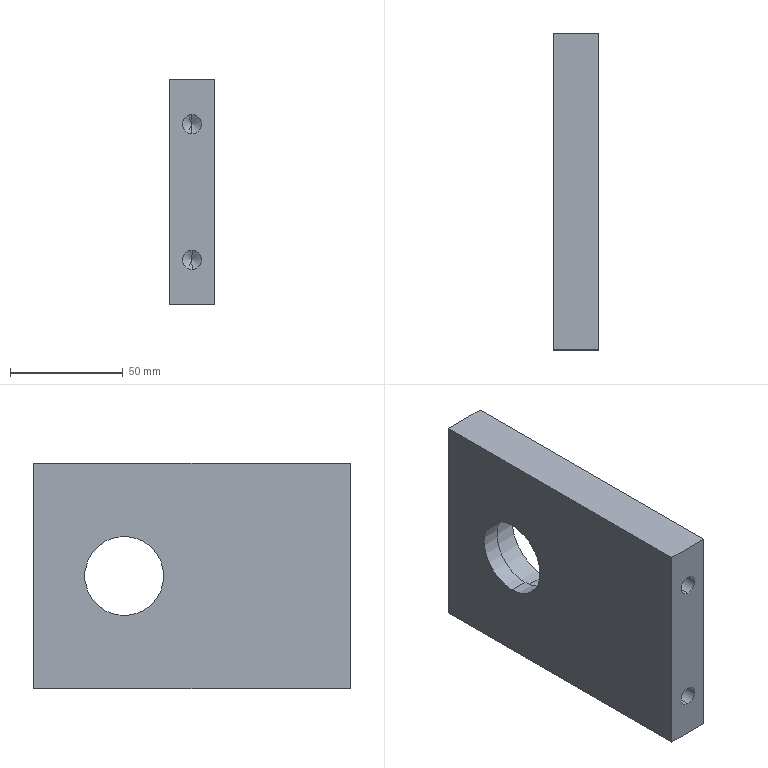Part | SolidWorks | features HoleWzd 2, ICE 2, Extrusion 1 | 1 solid | 27 faces | box 20 x 140 x 100 mm | volume 253738 mm3 | cylinder 12 | cone 8 | plane 7 | commonest cylinder face diameters 5 x4 8.5 x4 35 x2 40 x2
STEP:
#1=CARTESIAN_POINT('',(10.,55.,-32.5));
#2=VERTEX_POINT('',#1);
#3=CARTESIAN_POINT('',(10.,55.,-27.5));
#4=VERTEX_POINT('',#3);
#5=CARTESIAN_POINT('',(10.,55.,-30.));
#6=DIRECTION('',(0.,1.,0.));
#7=DIRECTION('',(0.,0.,1.));
#8=AXIS2_PLACEMENT_3D('',#5,#6,#7);
#9=CIRCLE('',#8,2.5);
#10=EDGE_CURVE('',#2,#4,#9,.T.);
#11=ORIENTED_EDGE('',*,*,#10,.F.);
#12=CARTESIAN_POINT('',(10.,70.,-32.5));
#13=VERTEX_POINT('',#12);
#14=CARTESIAN_POINT('',(10.,70.,-32.5));
#15=DIRECTION('',(0.,1.,0.));
#16=VECTOR('',#15,1000.);
#17=LINE('',#14,#16);
#18=EDGE_CURVE('',#2,#13,#17,.T.);
#19=ORIENTED_EDGE('',*,*,#18,.T.);
#20=CARTESIAN_POINT('',(10.,70.,-27.5));
#21=VERTEX_POINT('',#20);
#22=CARTESIAN_POINT('',(10.,70.,-30.));
#23=DIRECTION('',(0.,1.,0.));
#24=DIRECTION('',(0.,0.,1.));
#25=AXIS2_PLACEMENT_3D('',#22,#23,#24);
#26=CIRCLE('',#25,2.5);
#27=EDGE_CURVE('',#13,#21,#26,.T.);
#28=ORIENTED_EDGE('',*,*,#27,.T.);
#29=CARTESIAN_POINT('',(10.,70.,-27.5));
#30=DIRECTION('',(0.,1.,0.));
#31=VECTOR('',#30,1000.);
#32=LINE('',#29,#31);
#33=EDGE_CURVE('',#4,#21,#32,.T.);
#34=ORIENTED_EDGE('',*,*,#33,.F.);
#35=EDGE_LOOP('',(#11,#19,#28,#34));
#36=FACE_OUTER_BOUND('',#35,.T.);
#37=CARTESIAN_POINT('',(10.,70.,-30.));
#38=DIRECTION('',(0.,1.,0.));
#39=DIRECTION('',(0.,0.,1.));
#40=AXIS2_PLACEMENT_3D('',#37,#38,#39);
#41=CYLINDRICAL_SURFACE('',#40,2.5);
#42=ADVANCED_FACE('',(#36),#41,.F.);
#43=CARTESIAN_POINT('',(10.,53.498,-30.));
#44=VERTEX_POINT('',#43);
#45=CARTESIAN_POINT('',(10.,55.,-27.5));
#46=DIRECTION('',(0.,0.515,0.8572));
#47=VECTOR('',#46,1000.);
#48=LINE('',#45,#47);
#49=EDGE_CURVE('',#44,#4,#48,.T.);
#50=ORIENTED_EDGE('',*,*,#49,.F.);
#51=CARTESIAN_POINT('',(10.,55.,-32.5));
#52=DIRECTION('',(0.,0.515,-0.8572));
#53=VECTOR('',#52,1000.);
#54=LINE('',#51,#53);
#55=EDGE_CURVE('',#44,#2,#54,.T.);
#56=ORIENTED_EDGE('',*,*,#55,.T.);
#57=ORIENTED_EDGE('',*,*,#10,.T.);
#58=EDGE_LOOP('',(#50,#56,#57));
#59=FACE_OUTER_BOUND('',#58,.T.);
#60=CARTESIAN_POINT('',(10.,55.,-30.));
#61=DIRECTION('',(0.,1.,0.));
#62=DIRECTION('',(0.,0.,1.));
#63=AXIS2_PLACEMENT_3D('',#60,#61,#62);
#64=CONICAL_SURFACE('',#63,2.5,1.03);
#65=ADVANCED_FACE('',(#59),#64,.F.);
#66=CARTESIAN_POINT('',(10.,55.,27.5));
#67=VERTEX_POINT('',#66);
#68=CARTESIAN_POINT('',(10.,55.,32.5));
#69=VERTEX_POINT('',#68);
#70=CARTESIAN_POINT('',(10.,55.,30.));
#71=DIRECTION('',(0.,1.,0.));
#72=DIRECTION('',(0.,0.,1.));
#73=AXIS2_PLACEMENT_3D('',#70,#71,#72);
#74=CIRCLE('',#73,2.5);
#75=EDGE_CURVE('',#67,#69,#74,.T.);
#76=ORIENTED_EDGE('',*,*,#75,.F.);
#77=CARTESIAN_POINT('',(10.,70.,27.5));
#78=VERTEX_POINT('',#77);
#79=CARTESIAN_POINT('',(10.,70.,27.5));
#80=DIRECTION('',(0.,1.,0.));
#81=VECTOR('',#80,1000.);
#82=LINE('',#79,#81);
#83=EDGE_CURVE('',#67,#78,#82,.T.);
#84=ORIENTED_EDGE('',*,*,#83,.T.);
#85=CARTESIAN_POINT('',(10.,70.,32.5));
#86=VERTEX_POINT('',#85);
#87=CARTESIAN_POINT('',(10.,70.,30.));
#88=DIRECTION('',(0.,1.,0.));
#89=DIRECTION('',(0.,0.,1.));
#90=AXIS2_PLACEMENT_3D('',#87,#88,#89);
#91=CIRCLE('',#90,2.5);
#92=EDGE_CURVE('',#78,#86,#91,.T.);
#93=ORIENTED_EDGE('',*,*,#92,.T.);
#94=CARTESIAN_POINT('',(10.,70.,32.5));
#95=DIRECTION('',(0.,1.,0.));
#96=VECTOR('',#95,1000.);
#97=LINE('',#94,#96);
#98=EDGE_CURVE('',#69,#86,#97,.T.);
#99=ORIENTED_EDGE('',*,*,#98,.F.);
#100=EDGE_LOOP('',(#76,#84,#93,#99));
#101=FACE_OUTER_BOUND('',#100,.T.);
#102=CARTESIAN_POINT('',(10.,70.,30.));
#103=DIRECTION('',(0.,1.,0.));
#104=DIRECTION('',(0.,0.,1.));
#105=AXIS2_PLACEMENT_3D('',#102,#103,#104);
#106=CYLINDRICAL_SURFACE('',#105,2.5);
#107=ADVANCED_FACE('',(#101),#106,.F.);
#108=CARTESIAN_POINT('',(10.,53.498,30.));
#109=VERTEX_POINT('',#108);
#110=CARTESIAN_POINT('',(10.,55.,32.5));
#111=DIRECTION('',(0.,0.515,0.8572));
#112=VECTOR('',#111,1000.);
#113=LINE('',#110,#112);
#114=EDGE_CURVE('',#109,#69,#113,.T.);
#115=ORIENTED_EDGE('',*,*,#114,.F.);
#116=CARTESIAN_POINT('',(10.,55.,27.5));
#117=DIRECTION('',(0.,0.515,-0.8572));
#118=VECTOR('',#117,1000.);
#119=LINE('',#116,#118);
#120=EDGE_CURVE('',#109,#67,#119,.T.);
#121=ORIENTED_EDGE('',*,*,#120,.T.);
#122=ORIENTED_EDGE('',*,*,#75,.T.);
#123=EDGE_LOOP('',(#115,#121,#122));
#124=FACE_OUTER_BOUND('',#123,.T.);
#125=CARTESIAN_POINT('',(10.,55.,30.));
#126=DIRECTION('',(0.,1.,0.));
#127=DIRECTION('',(0.,0.,1.));
#128=AXIS2_PLACEMENT_3D('',#125,#126,#127);
#129=CONICAL_SURFACE('',#128,2.5,1.03);
#130=ADVANCED_FACE('',(#124),#129,.F.);
#131=CARTESIAN_POINT('',(0.,30.,17.5));
#132=VERTEX_POINT('',#131);
#133=CARTESIAN_POINT('',(0.,30.,-17.5));
#134=VERTEX_POINT('',#133);
#135=CARTESIAN_POINT('',(0.,30.,0.));
#136=DIRECTION('',(1.,0.,0.));
#137=DIRECTION('',(0.,0.,-1.));
#138=AXIS2_PLACEMENT_3D('',#135,#136,#137);
#139=CIRCLE('',#138,17.5);
#140=EDGE_CURVE('',#132,#134,#139,.T.);
#141=ORIENTED_EDGE('',*,*,#140,.F.);
#142=CARTESIAN_POINT('',(8.,30.,17.5));
#143=VERTEX_POINT('',#142);
#144=CARTESIAN_POINT('',(0.,30.,17.5));
#145=DIRECTION('',(1.,0.,0.));
#146=VECTOR('',#145,1000.);
#147=LINE('',#144,#146);
#148=EDGE_CURVE('',#132,#143,#147,.T.);
#149=ORIENTED_EDGE('',*,*,#148,.T.);
#150=CARTESIAN_POINT('',(8.,30.,-17.5));
#151=VERTEX_POINT('',#150);
#152=CARTESIAN_POINT('',(8.,30.,0.));
#153=DIRECTION('',(1.,0.,0.));
#154=DIRECTION('',(0.,0.,-1.));
#155=AXIS2_PLACEMENT_3D('',#152,#153,#154);
#156=CIRCLE('',#155,17.5);
#157=EDGE_CURVE('',#143,#151,#156,.T.);
#158=ORIENTED_EDGE('',*,*,#157,.T.);
#159=CARTESIAN_POINT('',(0.,30.,-17.5));
#160=DIRECTION('',(1.,0.,0.));
#161=VECTOR('',#160,1000.);
#162=LINE('',#159,#161);
#163=EDGE_CURVE('',#134,#151,#162,.T.);
#164=ORIENTED_EDGE('',*,*,#163,.F.);
#165=EDGE_LOOP('',(#141,#149,#158,#164));
#166=FACE_OUTER_BOUND('',#165,.T.);
#167=CARTESIAN_POINT('',(0.,30.,0.));
#168=DIRECTION('',(1.,0.,0.));
#169=DIRECTION('',(0.,0.,-1.));
#170=AXIS2_PLACEMENT_3D('',#167,#168,#169);
#171=CYLINDRICAL_SURFACE('',#170,17.5);
#172=ADVANCED_FACE('',(#166),#171,.F.);
#173=CARTESIAN_POINT('',(8.,30.,20.));
#174=VERTEX_POINT('',#173);
#175=CARTESIAN_POINT('',(8.,30.,-20.));
#176=VERTEX_POINT('',#175);
#177=CARTESIAN_POINT('',(8.,30.,0.));
#178=DIRECTION('',(1.,0.,0.));
#179=DIRECTION('',(0.,0.,-1.));
#180=AXIS2_PLACEMENT_3D('',#177,#178,#179);
#181=CIRCLE('',#180,20.);
#182=EDGE_CURVE('',#174,#176,#181,.T.);
#183=ORIENTED_EDGE('',*,*,#182,.F.);
#184=CARTESIAN_POINT('',(20.,30.,20.));
#185=VERTEX_POINT('',#184);
#186=CARTESIAN_POINT('',(8.,30.,20.));
#187=DIRECTION('',(1.,0.,0.));
#188=VECTOR('',#187,1000.);
#189=LINE('',#186,#188);
#190=EDGE_CURVE('',#174,#185,#189,.T.);
#191=ORIENTED_EDGE('',*,*,#190,.T.);
#192=CARTESIAN_POINT('',(20.,30.,-20.));
#193=VERTEX_POINT('',#192);
#194=CARTESIAN_POINT('',(20.,30.,0.));
#195=DIRECTION('',(1.,0.,0.));
#196=DIRECTION('',(0.,0.,-1.));
#197=AXIS2_PLACEMENT_3D('',#194,#195,#196);
#198=CIRCLE('',#197,20.);
#199=EDGE_CURVE('',#185,#193,#198,.T.);
#200=ORIENTED_EDGE('',*,*,#199,.T.);
#201=CARTESIAN_POINT('',(8.,30.,-20.));
#202=DIRECTION('',(1.,0.,0.));
#203=VECTOR('',#202,1000.);
#204=LINE('',#201,#203);
#205=EDGE_CURVE('',#176,#193,#204,.T.);
#206=ORIENTED_EDGE('',*,*,#205,.F.);
#207=EDGE_LOOP('',(#183,#191,#200,#206));
#208=FACE_OUTER_BOUND('',#207,.T.);
#209=CARTESIAN_POINT('',(8.,30.,0.));
#210=DIRECTION('',(1.,0.,0.));
#211=DIRECTION('',(0.,0.,-1.));
#212=AXIS2_PLACEMENT_3D('',#209,#210,#211);
#213=CYLINDRICAL_SURFACE('',#212,20.);
#214=ADVANCED_FACE('',(#208),#213,.F.);
#215=CARTESIAN_POINT('',(10.,-45.5,-25.75));
#216=VERTEX_POINT('',#215);
#217=CARTESIAN_POINT('',(10.,-45.5,-34.25));
#218=VERTEX_POINT('',#217);
#219=CARTESIAN_POINT('',(10.,-45.5,-30.));
#220=DIRECTION('',(0.,-1.,0.));
#221=DIRECTION('',(0.,0.,-1.));
#222=AXIS2_PLACEMENT_3D('',#219,#220,#221);
#223=CIRCLE('',#222,4.25);
#224=EDGE_CURVE('',#216,#218,#223,.T.);
#225=ORIENTED_EDGE('',*,*,#224,.F.);
#226=CARTESIAN_POINT('',(10.,-70.,-25.75));
#227=VERTEX_POINT('',#226);
#228=CARTESIAN_POINT('',(10.,-70.,-25.75));
#229=DIRECTION('',(0.,-1.,0.));
#230=VECTOR('',#229,1000.);
#231=LINE('',#228,#230);
#232=EDGE_CURVE('',#216,#227,#231,.T.);
#233=ORIENTED_EDGE('',*,*,#232,.T.);
#234=CARTESIAN_POINT('',(10.,-70.,-34.25));
#235=VERTEX_POINT('',#234);
#236=CARTESIAN_POINT('',(10.,-70.,-30.));
#237=DIRECTION('',(0.,-1.,0.));
#238=DIRECTION('',(0.,0.,-1.));
#239=AXIS2_PLACEMENT_3D('',#236,#237,#238);
#240=CIRCLE('',#239,4.25);
#241=EDGE_CURVE('',#227,#235,#240,.T.);
#242=ORIENTED_EDGE('',*,*,#241,.T.);
#243=CARTESIAN_POINT('',(10.,-70.,-34.25));
#244=DIRECTION('',(0.,-1.,0.));
#245=VECTOR('',#244,1000.);
#246=LINE('',#243,#245);
#247=EDGE_CURVE('',#218,#235,#246,.T.);
#248=ORIENTED_EDGE('',*,*,#247,.F.);
#249=EDGE_LOOP('',(#225,#233,#242,#248));
#250=FACE_OUTER_BOUND('',#249,.T.);
#251=CARTESIAN_POINT('',(10.,-70.,-30.));
#252=DIRECTION('',(0.,-1.,0.));
#253=DIRECTION('',(0.,0.,-1.));
#254=AXIS2_PLACEMENT_3D('',#251,#252,#253);
#255=CYLINDRICAL_SURFACE('',#254,4.25);
#256=ADVANCED_FACE('',(#250),#255,.F.);
#257=CARTESIAN_POINT('',(10.,-42.946,-30.));
#258=VERTEX_POINT('',#257);
#259=CARTESIAN_POINT('',(10.,-45.5,-34.25));
#260=DIRECTION('',(0.,-0.515,-0.8572));
#261=VECTOR('',#260,1000.);
#262=LINE('',#259,#261);
#263=EDGE_CURVE('',#258,#218,#262,.T.);
#264=ORIENTED_EDGE('',*,*,#263,.F.);
#265=CARTESIAN_POINT('',(10.,-45.5,-25.75));
#266=DIRECTION('',(0.,-0.515,0.8572));
#267=VECTOR('',#266,1000.);
#268=LINE('',#265,#267);
#269=EDGE_CURVE('',#258,#216,#268,.T.);
#270=ORIENTED_EDGE('',*,*,#269,.T.);
#271=ORIENTED_EDGE('',*,*,#224,.T.);
#272=EDGE_LOOP('',(#264,#270,#271));
#273=FACE_OUTER_BOUND('',#272,.T.);
#274=CARTESIAN_POINT('',(10.,-45.5,-30.));
#275=DIRECTION('',(0.,-1.,0.));
#276=DIRECTION('',(0.,0.,-1.));
#277=AXIS2_PLACEMENT_3D('',#274,#275,#276);
#278=CONICAL_SURFACE('',#277,4.25,1.03);
#279=ADVANCED_FACE('',(#273),#278,.F.);
#280=CARTESIAN_POINT('',(10.,-45.5,34.25));
#281=VERTEX_POINT('',#280);
#282=CARTESIAN_POINT('',(10.,-45.5,25.75));
#283=VERTEX_POINT('',#282);
#284=CARTESIAN_POINT('',(10.,-45.5,30.));
#285=DIRECTION('',(0.,-1.,0.));
#286=DIRECTION('',(0.,0.,-1.));
#287=AXIS2_PLACEMENT_3D('',#284,#285,#286);
#288=CIRCLE('',#287,4.25);
#289=EDGE_CURVE('',#281,#283,#288,.T.);
#290=ORIENTED_EDGE('',*,*,#289,.F.);
#291=CARTESIAN_POINT('',(10.,-70.,34.25));
#292=VERTEX_POINT('',#291);
#293=CARTESIAN_POINT('',(10.,-70.,34.25));
#294=DIRECTION('',(0.,-1.,0.));
#295=VECTOR('',#294,1000.);
#296=LINE('',#293,#295);
#297=EDGE_CURVE('',#281,#292,#296,.T.);
#298=ORIENTED_EDGE('',*,*,#297,.T.);
#299=CARTESIAN_POINT('',(10.,-70.,25.75));
#300=VERTEX_POINT('',#299);
#301=CARTESIAN_POINT('',(10.,-70.,30.));
#302=DIRECTION('',(0.,-1.,0.));
#303=DIRECTION('',(0.,0.,-1.));
#304=AXIS2_PLACEMENT_3D('',#301,#302,#303);
#305=CIRCLE('',#304,4.25);
#306=EDGE_CURVE('',#292,#300,#305,.T.);
#307=ORIENTED_EDGE('',*,*,#306,.T.);
#308=CARTESIAN_POINT('',(10.,-70.,25.75));
#309=DIRECTION('',(0.,-1.,0.));
#310=VECTOR('',#309,1000.);
#311=LINE('',#308,#310);
#312=EDGE_CURVE('',#283,#300,#311,.T.);
#313=ORIENTED_EDGE('',*,*,#312,.F.);
#314=EDGE_LOOP('',(#290,#298,#307,#313));
#315=FACE_OUTER_BOUND('',#314,.T.);
#316=CARTESIAN_POINT('',(10.,-70.,30.));
#317=DIRECTION('',(0.,-1.,0.));
#318=DIRECTION('',(0.,0.,-1.));
#319=AXIS2_PLACEMENT_3D('',#316,#317,#318);
#320=CYLINDRICAL_SURFACE('',#319,4.25);
#321=ADVANCED_FACE('',(#315),#320,.F.);
#322=CARTESIAN_POINT('',(10.,-42.946,30.));
#323=VERTEX_POINT('',#322);
#324=CARTESIAN_POINT('',(10.,-45.5,25.75));
#325=DIRECTION('',(0.,-0.515,-0.8572));
#326=VECTOR('',#325,1000.);
#327=LINE('',#324,#326);
#328=EDGE_CURVE('',#323,#283,#327,.T.);
#329=ORIENTED_EDGE('',*,*,#328,.F.);
#330=CARTESIAN_POINT('',(10.,-45.5,34.25));
#331=DIRECTION('',(0.,-0.515,0.8572));
#332=VECTOR('',#331,1000.);
#333=LINE('',#330,#332);
#334=EDGE_CURVE('',#323,#281,#333,.T.);
#335=ORIENTED_EDGE('',*,*,#334,.T.);
#336=ORIENTED_EDGE('',*,*,#289,.T.);
#337=EDGE_LOOP('',(#329,#335,#336));
#338=FACE_OUTER_BOUND('',#337,.T.);
#339=CARTESIAN_POINT('',(10.,-45.5,30.));
#340=DIRECTION('',(0.,-1.,0.));
#341=DIRECTION('',(0.,0.,-1.));
#342=AXIS2_PLACEMENT_3D('',#339,#340,#341);
#343=CONICAL_SURFACE('',#342,4.25,1.03);
#344=ADVANCED_FACE('',(#338),#343,.F.);
#345=CARTESIAN_POINT('',(0.,-70.,-50.));
#346=VERTEX_POINT('',#345);
#347=CARTESIAN_POINT('',(0.,70.,-50.));
#348=VERTEX_POINT('',#347);
#349=CARTESIAN_POINT('',(0.,70.,-50.));
#350=DIRECTION('',(0.,1.,0.));
#351=VECTOR('',#350,1000.);
#352=LINE('',#349,#351);
#353=EDGE_CURVE('',#346,#348,#352,.T.);
#354=ORIENTED_EDGE('',*,*,#353,.T.);
#355=CARTESIAN_POINT('',(20.,70.,-50.));
#356=VERTEX_POINT('',#355);
#357=CARTESIAN_POINT('',(20.,70.,-50.));
#358=DIRECTION('',(-1.,0.,0.));
#359=VECTOR('',#358,1000.);
#360=LINE('',#357,#359);
#361=EDGE_CURVE('',#356,#348,#360,.T.);
#362=ORIENTED_EDGE('',*,*,#361,.F.);
#363=CARTESIAN_POINT('',(20.,-70.,-50.));
#364=VERTEX_POINT('',#363);
#365=CARTESIAN_POINT('',(20.,70.,-50.));
#366=DIRECTION('',(0.,1.,0.));
#367=VECTOR('',#366,1000.);
#368=LINE('',#365,#367);
#369=EDGE_CURVE('',#364,#356,#368,.T.);
#370=ORIENTED_EDGE('',*,*,#369,.F.);
#371=CARTESIAN_POINT('',(20.,-70.,-50.));
#372=DIRECTION('',(-1.,0.,0.));
#373=VECTOR('',#372,1000.);
#374=LINE('',#371,#373);
#375=EDGE_CURVE('',#364,#346,#374,.T.);
#376=ORIENTED_EDGE('',*,*,#375,.T.);
#377=EDGE_LOOP('',(#354,#362,#370,#376));
#378=FACE_OUTER_BOUND('',#377,.T.);
#379=CARTESIAN_POINT('',(20.,70.,-50.));
#380=DIRECTION('',(0.,0.,1.));
#381=DIRECTION('',(0.,-1.,0.));
#382=AXIS2_PLACEMENT_3D('',#379,#380,#381);
#383=PLANE('',#382);
#384=ADVANCED_FACE('',(#378),#383,.F.);
#385=CARTESIAN_POINT('',(10.,70.,-30.));
#386=DIRECTION('',(0.,1.,0.));
#387=DIRECTION('',(0.,0.,1.));
#388=AXIS2_PLACEMENT_3D('',#385,#386,#387);
#389=CIRCLE('',#388,2.5);
#390=EDGE_CURVE('',#21,#13,#389,.T.);
#391=ORIENTED_EDGE('',*,*,#390,.F.);
#392=ORIENTED_EDGE('',*,*,#27,.F.);
#393=EDGE_LOOP('',(#391,#392));
#394=FACE_BOUND('',#393,.T.);
#395=CARTESIAN_POINT('',(10.,70.,30.));
#396=DIRECTION('',(0.,1.,0.));
#397=DIRECTION('',(0.,0.,1.));
#398=AXIS2_PLACEMENT_3D('',#395,#396,#397);
#399=CIRCLE('',#398,2.5);
#400=EDGE_CURVE('',#86,#78,#399,.T.);
#401=ORIENTED_EDGE('',*,*,#400,.F.);
#402=ORIENTED_EDGE('',*,*,#92,.F.);
#403=EDGE_LOOP('',(#401,#402));
#404=FACE_BOUND('',#403,.T.);
#405=CARTESIAN_POINT('',(0.,70.,50.));
#406=VERTEX_POINT('',#405);
#407=CARTESIAN_POINT('',(0.,70.,50.));
#408=DIRECTION('',(0.,0.,1.));
#409=VECTOR('',#408,1000.);
#410=LINE('',#407,#409);
#411=EDGE_CURVE('',#348,#406,#410,.T.);
#412=ORIENTED_EDGE('',*,*,#411,.T.);
#413=CARTESIAN_POINT('',(20.,70.,50.));
#414=VERTEX_POINT('',#413);
#415=CARTESIAN_POINT('',(20.,70.,50.));
#416=DIRECTION('',(-1.,0.,0.));
#417=VECTOR('',#416,1000.);
#418=LINE('',#415,#417);
#419=EDGE_CURVE('',#414,#406,#418,.T.);
#420=ORIENTED_EDGE('',*,*,#419,.F.);
#421=CARTESIAN_POINT('',(20.,70.,50.));
#422=DIRECTION('',(0.,0.,1.));
#423=VECTOR('',#422,1000.);
#424=LINE('',#421,#423);
#425=EDGE_CURVE('',#356,#414,#424,.T.);
#426=ORIENTED_EDGE('',*,*,#425,.F.);
#427=ORIENTED_EDGE('',*,*,#361,.T.);
#428=EDGE_LOOP('',(#412,#420,#426,#427));
#429=FACE_OUTER_BOUND('',#428,.T.);
#430=CARTESIAN_POINT('',(20.,70.,50.));
#431=DIRECTION('',(0.,-1.,0.));
#432=DIRECTION('',(0.,0.,-1.));
#433=AXIS2_PLACEMENT_3D('',#430,#431,#432);
#434=PLANE('',#433);
#435=ADVANCED_FACE('',(#394,#404,#429),#434,.F.);
#436=CARTESIAN_POINT('',(0.,-70.,50.));
#437=VERTEX_POINT('',#436);
#438=CARTESIAN_POINT('',(0.,70.,50.));
#439=DIRECTION('',(0.,-1.,0.));
#440=VECTOR('',#439,1000.);
#441=LINE('',#438,#440);
#442=EDGE_CURVE('',#406,#437,#441,.T.);
#443=ORIENTED_EDGE('',*,*,#442,.T.);
#444=CARTESIAN_POINT('',(20.,-70.,50.));
#445=VERTEX_POINT('',#444);
#446=CARTESIAN_POINT('',(20.,-70.,50.));
#447=DIRECTION('',(-1.,0.,0.));
#448=VECTOR('',#447,1000.);
#449=LINE('',#446,#448);
#450=EDGE_CURVE('',#445,#437,#449,.T.);
#451=ORIENTED_EDGE('',*,*,#450,.F.);
#452=CARTESIAN_POINT('',(20.,70.,50.));
#453=DIRECTION('',(0.,-1.,0.));
#454=VECTOR('',#453,1000.);
#455=LINE('',#452,#454);
#456=EDGE_CURVE('',#414,#445,#455,.T.);
#457=ORIENTED_EDGE('',*,*,#456,.F.);
#458=ORIENTED_EDGE('',*,*,#419,.T.);
#459=EDGE_LOOP('',(#443,#451,#457,#458));
#460=FACE_OUTER_BOUND('',#459,.T.);
#461=CARTESIAN_POINT('',(20.,70.,50.));
#462=DIRECTION('',(0.,0.,-1.));
#463=DIRECTION('',(0.,1.,0.));
#464=AXIS2_PLACEMENT_3D('',#461,#462,#463);
#465=PLANE('',#464);
#466=ADVANCED_FACE('',(#460),#465,.F.);
#467=CARTESIAN_POINT('',(10.,-70.,-30.));
#468=DIRECTION('',(0.,-1.,0.));
#469=DIRECTION('',(0.,0.,-1.));
#470=AXIS2_PLACEMENT_3D('',#467,#468,#469);
#471=CIRCLE('',#470,4.25);
#472=EDGE_CURVE('',#235,#227,#471,.T.);
#473=ORIENTED_EDGE('',*,*,#472,.F.);
#474=ORIENTED_EDGE('',*,*,#241,.F.);
#475=EDGE_LOOP('',(#473,#474));
#476=FACE_BOUND('',#475,.T.);
#477=CARTESIAN_POINT('',(10.,-70.,30.));
#478=DIRECTION('',(0.,-1.,0.));
#479=DIRECTION('',(0.,0.,-1.));
#480=AXIS2_PLACEMENT_3D('',#477,#478,#479);
#481=CIRCLE('',#480,4.25);
#482=EDGE_CURVE('',#300,#292,#481,.T.);
#483=ORIENTED_EDGE('',*,*,#482,.F.);
#484=ORIENTED_EDGE('',*,*,#306,.F.);
#485=EDGE_LOOP('',(#483,#484));
#486=FACE_BOUND('',#485,.T.);
#487=CARTESIAN_POINT('',(0.,-70.,50.));
#488=DIRECTION('',(0.,0.,-1.));
#489=VECTOR('',#488,1000.);
#490=LINE('',#487,#489);
#491=EDGE_CURVE('',#437,#346,#490,.T.);
#492=ORIENTED_EDGE('',*,*,#491,.T.);
#493=ORIENTED_EDGE('',*,*,#375,.F.);
#494=CARTESIAN_POINT('',(20.,-70.,50.));
#495=DIRECTION('',(0.,0.,-1.));
#496=VECTOR('',#495,1000.);
#497=LINE('',#494,#496);
#498=EDGE_CURVE('',#445,#364,#497,.T.);
#499=ORIENTED_EDGE('',*,*,#498,.F.);
#500=ORIENTED_EDGE('',*,*,#450,.T.);
#501=EDGE_LOOP('',(#492,#493,#499,#500));
#502=FACE_OUTER_BOUND('',#501,.T.);
#503=CARTESIAN_POINT('',(20.,-70.,50.));
#504=DIRECTION('',(0.,1.,0.));
#505=DIRECTION('',(0.,0.,1.));
#506=AXIS2_PLACEMENT_3D('',#503,#504,#505);
#507=PLANE('',#506);
#508=ADVANCED_FACE('',(#476,#486,#502),#507,.F.);
#509=CARTESIAN_POINT('',(20.,30.,0.));
#510=DIRECTION('',(1.,0.,0.));
#511=DIRECTION('',(0.,0.,-1.));
#512=AXIS2_PLACEMENT_3D('',#509,#510,#511);
#513=CIRCLE('',#512,20.);
#514=EDGE_CURVE('',#193,#185,#513,.T.);
#515=ORIENTED_EDGE('',*,*,#514,.F.);
#516=ORIENTED_EDGE('',*,*,#199,.F.);
#517=EDGE_LOOP('',(#515,#516));
#518=FACE_BOUND('',#517,.T.);
#519=ORIENTED_EDGE('',*,*,#369,.T.);
#520=ORIENTED_EDGE('',*,*,#425,.T.);
#521=ORIENTED_EDGE('',*,*,#456,.T.);
#522=ORIENTED_EDGE('',*,*,#498,.T.);
#523=EDGE_LOOP('',(#519,#520,#521,#522));
#524=FACE_OUTER_BOUND('',#523,.T.);
#525=CARTESIAN_POINT('',(20.,0.,0.));
#526=DIRECTION('',(1.,0.,0.));
#527=DIRECTION('',(0.,0.,-1.));
#528=AXIS2_PLACEMENT_3D('',#525,#526,#527);
#529=PLANE('',#528);
#530=ADVANCED_FACE('',(#518,#524),#529,.T.);
#531=CARTESIAN_POINT('',(0.,30.,0.));
#532=DIRECTION('',(1.,0.,0.));
#533=DIRECTION('',(0.,0.,-1.));
#534=AXIS2_PLACEMENT_3D('',#531,#532,#533);
#535=CIRCLE('',#534,17.5);
#536=EDGE_CURVE('',#134,#132,#535,.T.);
#537=ORIENTED_EDGE('',*,*,#536,.T.);
#538=ORIENTED_EDGE('',*,*,#140,.T.);
#539=EDGE_LOOP('',(#537,#538));
#540=FACE_BOUND('',#539,.T.);
#541=ORIENTED_EDGE('',*,*,#353,.F.);
#542=ORIENTED_EDGE('',*,*,#491,.F.);
#543=ORIENTED_EDGE('',*,*,#442,.F.);
#544=ORIENTED_EDGE('',*,*,#411,.F.);
#545=EDGE_LOOP('',(#541,#542,#543,#544));
#546=FACE_OUTER_BOUND('',#545,.T.);
#547=CARTESIAN_POINT('',(0.,0.,0.));
#548=DIRECTION('',(1.,0.,0.));
#549=DIRECTION('',(0.,0.,-1.));
#550=AXIS2_PLACEMENT_3D('',#547,#548,#549);
#551=PLANE('',#550);
#552=ADVANCED_FACE('',(#540,#546),#551,.F.);
#553=ORIENTED_EDGE('',*,*,#334,.F.);
#554=ORIENTED_EDGE('',*,*,#328,.T.);
#555=CARTESIAN_POINT('',(10.,-45.5,30.));
#556=DIRECTION('',(0.,-1.,0.));
#557=DIRECTION('',(0.,0.,-1.));
#558=AXIS2_PLACEMENT_3D('',#555,#556,#557);
#559=CIRCLE('',#558,4.25);
#560=EDGE_CURVE('',#283,#281,#559,.T.);
#561=ORIENTED_EDGE('',*,*,#560,.T.);
#562=EDGE_LOOP('',(#553,#554,#561));
#563=FACE_OUTER_BOUND('',#562,.T.);
#564=CARTESIAN_POINT('',(10.,-45.5,30.));
#565=DIRECTION('',(0.,-1.,0.));
#566=DIRECTION('',(0.,0.,-1.));
#567=AXIS2_PLACEMENT_3D('',#564,#565,#566);
#568=CONICAL_SURFACE('',#567,4.25,1.03);
#569=ADVANCED_FACE('',(#563),#568,.F.);
#570=ORIENTED_EDGE('',*,*,#297,.F.);
#571=ORIENTED_EDGE('',*,*,#560,.F.);
#572=ORIENTED_EDGE('',*,*,#312,.T.);
#573=ORIENTED_EDGE('',*,*,#482,.T.);
#574=EDGE_LOOP('',(#570,#571,#572,#573));
#575=FACE_OUTER_BOUND('',#574,.T.);
#576=CARTESIAN_POINT('',(10.,-70.,30.));
#577=DIRECTION('',(0.,-1.,0.));
#578=DIRECTION('',(0.,0.,-1.));
#579=AXIS2_PLACEMENT_3D('',#576,#577,#578);
#580=CYLINDRICAL_SURFACE('',#579,4.25);
#581=ADVANCED_FACE('',(#575),#580,.F.);
#582=ORIENTED_EDGE('',*,*,#269,.F.);
#583=ORIENTED_EDGE('',*,*,#263,.T.);
#584=CARTESIAN_POINT('',(10.,-45.5,-30.));
#585=DIRECTION('',(0.,-1.,0.));
#586=DIRECTION('',(0.,0.,-1.));
#587=AXIS2_PLACEMENT_3D('',#584,#585,#586);
#588=CIRCLE('',#587,4.25);
#589=EDGE_CURVE('',#218,#216,#588,.T.);
#590=ORIENTED_EDGE('',*,*,#589,.T.);
#591=EDGE_LOOP('',(#582,#583,#590));
#592=FACE_OUTER_BOUND('',#591,.T.);
#593=CARTESIAN_POINT('',(10.,-45.5,-30.));
#594=DIRECTION('',(0.,-1.,0.));
#595=DIRECTION('',(0.,0.,-1.));
#596=AXIS2_PLACEMENT_3D('',#593,#594,#595);
#597=CONICAL_SURFACE('',#596,4.25,1.03);
#598=ADVANCED_FACE('',(#592),#597,.F.);
#599=ORIENTED_EDGE('',*,*,#232,.F.);
#600=ORIENTED_EDGE('',*,*,#589,.F.);
#601=ORIENTED_EDGE('',*,*,#247,.T.);
#602=ORIENTED_EDGE('',*,*,#472,.T.);
#603=EDGE_LOOP('',(#599,#600,#601,#602));
#604=FACE_OUTER_BOUND('',#603,.T.);
#605=CARTESIAN_POINT('',(10.,-70.,-30.));
#606=DIRECTION('',(0.,-1.,0.));
#607=DIRECTION('',(0.,0.,-1.));
#608=AXIS2_PLACEMENT_3D('',#605,#606,#607);
#609=CYLINDRICAL_SURFACE('',#608,4.25);
#610=ADVANCED_FACE('',(#604),#609,.F.);
#611=ORIENTED_EDGE('',*,*,#190,.F.);
#612=CARTESIAN_POINT('',(8.,30.,0.));
#613=DIRECTION('',(1.,0.,0.));
#614=DIRECTION('',(0.,0.,-1.));
#615=AXIS2_PLACEMENT_3D('',#612,#613,#614);
#616=CIRCLE('',#615,20.);
#617=EDGE_CURVE('',#176,#174,#616,.T.);
#618=ORIENTED_EDGE('',*,*,#617,.F.);
#619=ORIENTED_EDGE('',*,*,#205,.T.);
#620=ORIENTED_EDGE('',*,*,#514,.T.);
#621=EDGE_LOOP('',(#611,#618,#619,#620));
#622=FACE_OUTER_BOUND('',#621,.T.);
#623=CARTESIAN_POINT('',(8.,30.,0.));
#624=DIRECTION('',(1.,0.,0.));
#625=DIRECTION('',(0.,0.,-1.));
#626=AXIS2_PLACEMENT_3D('',#623,#624,#625);
#627=CYLINDRICAL_SURFACE('',#626,20.);
#628=ADVANCED_FACE('',(#622),#627,.F.);
#629=CARTESIAN_POINT('',(8.,30.,0.));
#630=DIRECTION('',(1.,0.,0.));
#631=DIRECTION('',(0.,0.,-1.));
#632=AXIS2_PLACEMENT_3D('',#629,#630,#631);
#633=CIRCLE('',#632,17.5);
#634=EDGE_CURVE('',#151,#143,#633,.T.);
#635=ORIENTED_EDGE('',*,*,#634,.F.);
#636=ORIENTED_EDGE('',*,*,#157,.F.);
#637=EDGE_LOOP('',(#635,#636));
#638=FACE_BOUND('',#637,.T.);
#639=ORIENTED_EDGE('',*,*,#617,.T.);
#640=ORIENTED_EDGE('',*,*,#182,.T.);
#641=EDGE_LOOP('',(#639,#640));
#642=FACE_OUTER_BOUND('',#641,.T.);
#643=CARTESIAN_POINT('',(8.,30.,0.));
#644=DIRECTION('',(1.,0.,0.));
#645=DIRECTION('',(0.,0.,-1.));
#646=AXIS2_PLACEMENT_3D('',#643,#644,#645);
#647=PLANE('',#646);
#648=ADVANCED_FACE('',(#638,#642),#647,.T.);
#649=ORIENTED_EDGE('',*,*,#148,.F.);
#650=ORIENTED_EDGE('',*,*,#536,.F.);
#651=ORIENTED_EDGE('',*,*,#163,.T.);
#652=ORIENTED_EDGE('',*,*,#634,.T.);
#653=EDGE_LOOP('',(#649,#650,#651,#652));
#654=FACE_OUTER_BOUND('',#653,.T.);
#655=CARTESIAN_POINT('',(0.,30.,0.));
#656=DIRECTION('',(1.,0.,0.));
#657=DIRECTION('',(0.,0.,-1.));
#658=AXIS2_PLACEMENT_3D('',#655,#656,#657);
#659=CYLINDRICAL_SURFACE('',#658,17.5);
#660=ADVANCED_FACE('',(#654),#659,.F.);
#661=ORIENTED_EDGE('',*,*,#120,.F.);
#662=ORIENTED_EDGE('',*,*,#114,.T.);
#663=CARTESIAN_POINT('',(10.,55.,30.));
#664=DIRECTION('',(0.,1.,0.));
#665=DIRECTION('',(0.,0.,1.));
#666=AXIS2_PLACEMENT_3D('',#663,#664,#665);
#667=CIRCLE('',#666,2.5);
#668=EDGE_CURVE('',#69,#67,#667,.T.);
#669=ORIENTED_EDGE('',*,*,#668,.T.);
#670=EDGE_LOOP('',(#661,#662,#669));
#671=FACE_OUTER_BOUND('',#670,.T.);
#672=CARTESIAN_POINT('',(10.,55.,30.));
#673=DIRECTION('',(0.,1.,0.));
#674=DIRECTION('',(0.,0.,1.));
#675=AXIS2_PLACEMENT_3D('',#672,#673,#674);
#676=CONICAL_SURFACE('',#675,2.5,1.03);
#677=ADVANCED_FACE('',(#671),#676,.F.);
#678=ORIENTED_EDGE('',*,*,#83,.F.);
#679=ORIENTED_EDGE('',*,*,#668,.F.);
#680=ORIENTED_EDGE('',*,*,#98,.T.);
#681=ORIENTED_EDGE('',*,*,#400,.T.);
#682=EDGE_LOOP('',(#678,#679,#680,#681));
#683=FACE_OUTER_BOUND('',#682,.T.);
#684=CARTESIAN_POINT('',(10.,70.,30.));
#685=DIRECTION('',(0.,1.,0.));
#686=DIRECTION('',(0.,0.,1.));
#687=AXIS2_PLACEMENT_3D('',#684,#685,#686);
#688=CYLINDRICAL_SURFACE('',#687,2.5);
#689=ADVANCED_FACE('',(#683),#688,.F.);
#690=ORIENTED_EDGE('',*,*,#55,.F.);
#691=ORIENTED_EDGE('',*,*,#49,.T.);
#692=CARTESIAN_POINT('',(10.,55.,-30.));
#693=DIRECTION('',(0.,1.,0.));
#694=DIRECTION('',(0.,0.,1.));
#695=AXIS2_PLACEMENT_3D('',#692,#693,#694);
#696=CIRCLE('',#695,2.5);
#697=EDGE_CURVE('',#4,#2,#696,.T.);
#698=ORIENTED_EDGE('',*,*,#697,.T.);
#699=EDGE_LOOP('',(#690,#691,#698));
#700=FACE_OUTER_BOUND('',#699,.T.);
#701=CARTESIAN_POINT('',(10.,55.,-30.));
#702=DIRECTION('',(0.,1.,0.));
#703=DIRECTION('',(0.,0.,1.));
#704=AXIS2_PLACEMENT_3D('',#701,#702,#703);
#705=CONICAL_SURFACE('',#704,2.5,1.03);
#706=ADVANCED_FACE('',(#700),#705,.F.);
#707=ORIENTED_EDGE('',*,*,#18,.F.);
#708=ORIENTED_EDGE('',*,*,#697,.F.);
#709=ORIENTED_EDGE('',*,*,#33,.T.);
#710=ORIENTED_EDGE('',*,*,#390,.T.);
#711=EDGE_LOOP('',(#707,#708,#709,#710));
#712=FACE_OUTER_BOUND('',#711,.T.);
#713=CARTESIAN_POINT('',(10.,70.,-30.));
#714=DIRECTION('',(0.,1.,0.));
#715=DIRECTION('',(0.,0.,1.));
#716=AXIS2_PLACEMENT_3D('',#713,#714,#715);
#717=CYLINDRICAL_SURFACE('',#716,2.5);
#718=ADVANCED_FACE('',(#712),#717,.F.);
#719=CLOSED_SHELL('',(#42,#65,#107,#130,#172,#214,#256,#279,#321,#344,#384,#435,#466,#508,#530,#552,#569,#581,#598,#610,#628,#648,#660,#677,#689,#706,#718));
#720=MANIFOLD_SOLID_BREP('',#719);
#721=CARTESIAN_POINT('',(0.,0.,0.));
#722=DIRECTION('',(0.,0.,1.));
#723=DIRECTION('',(1.,0.,0.));
#724=AXIS2_PLACEMENT_3D('',#721,#722,#723);
#725=(LENGTH_UNIT()NAMED_UNIT(*)SI_UNIT(.MILLI.,.METRE.));
#726=UNCERTAINTY_MEASURE_WITH_UNIT(LENGTH_MEASURE(0.00001),#725,'','');
#727=(NAMED_UNIT(*)PLANE_ANGLE_UNIT()SI_UNIT($,.RADIAN.));
#728=(NAMED_UNIT(*)SI_UNIT($,.STERADIAN.)SOLID_ANGLE_UNIT());
#729=(GEOMETRIC_REPRESENTATION_CONTEXT(3)GLOBAL_UNCERTAINTY_ASSIGNED_CONTEXT((#726))GLOBAL_UNIT_ASSIGNED_CONTEXT((#725,#727,#728))REPRESENTATION_CONTEXT('',''));
#730=ADVANCED_BREP_SHAPE_REPRESENTATION('',(#720,#724),#729);